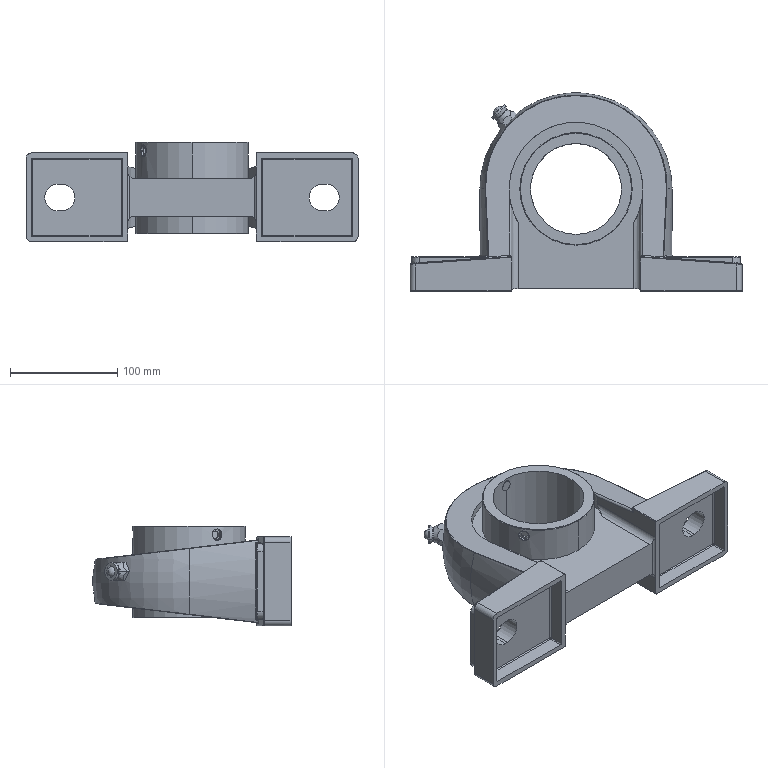Part | SolidWorks | features ICE 13, Fillet 12, Draft 4, RevCut 2, Revolution 2, 3DProfileFeature 1, Chamfer 1, CirPattern 1, HoleWzd 1, RefAxis 1 | 1 solid | 251 faces | box 310 x 184.907 x 93.1 mm | volume 1419775 mm3 | cylinder 96 | plane 68 | spline 46 | cone 16 | torus 15 | sphere 10 | commonest cylinder face diameters 1 x22 2 x16 10 x12 4 x10 3 x8 125 x6